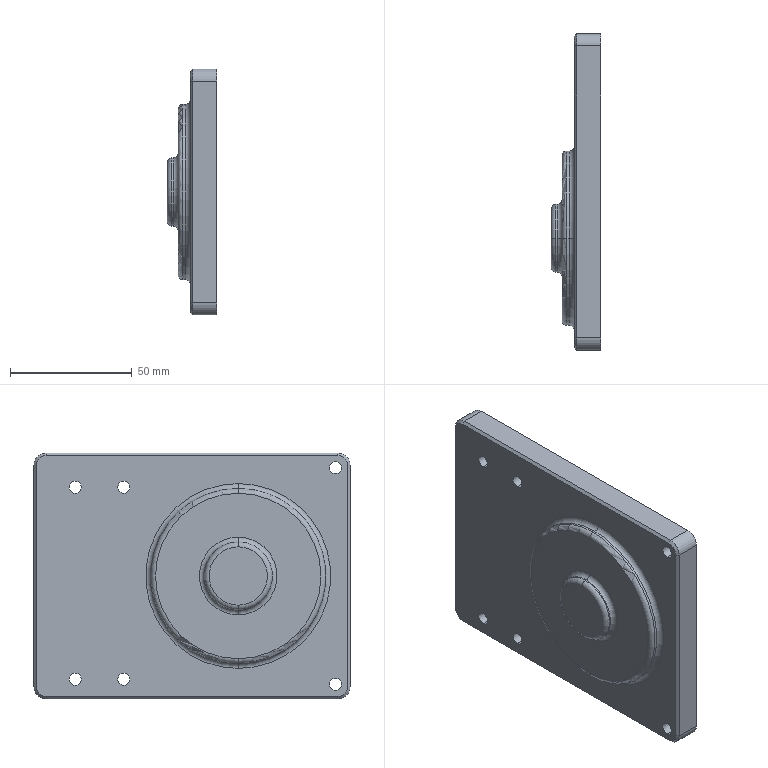Part | SolidWorks | features ICE 9, Fillet 4, Chamfer 1, Extrusion 1, HoleWzd 1 | 1 solid | 85 faces | box 20.5 x 130 x 101 mm | volume 69425 mm3 | cylinder 37 | plane 32 | torus 8 | cone 8 | commonest cylinder face diameters 5 x12 10 x7 8 x4 18 x2 20 x2 22 x2